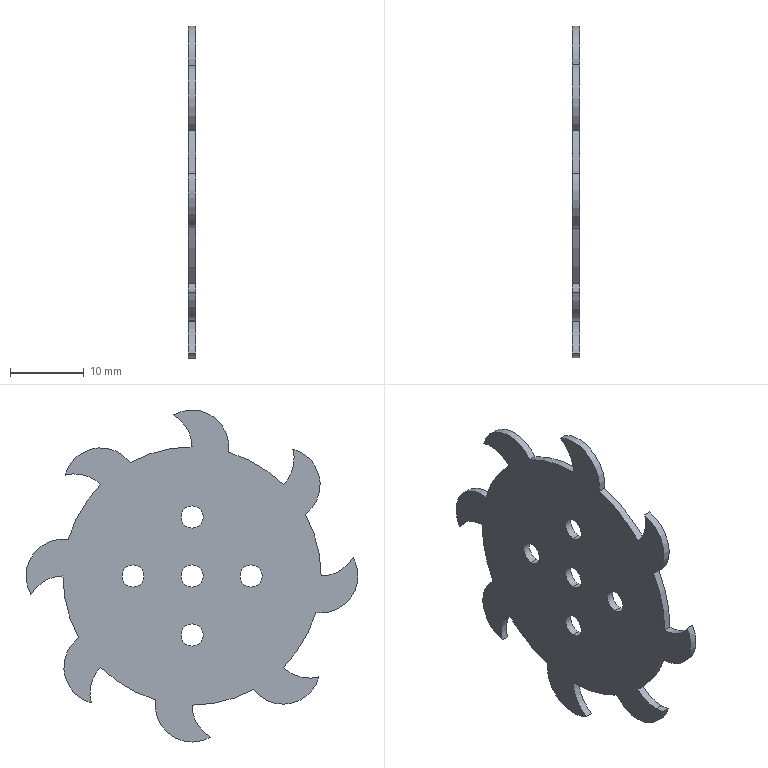Part | STEP file | Cutting knife | 1 solid | 40 faces | box 1 x 45 x 45 mm | volume 1128 mm3 | cylinder 38 | plane 2 | commonest cylinder face diameters 10 x20 3 x10 35 x8